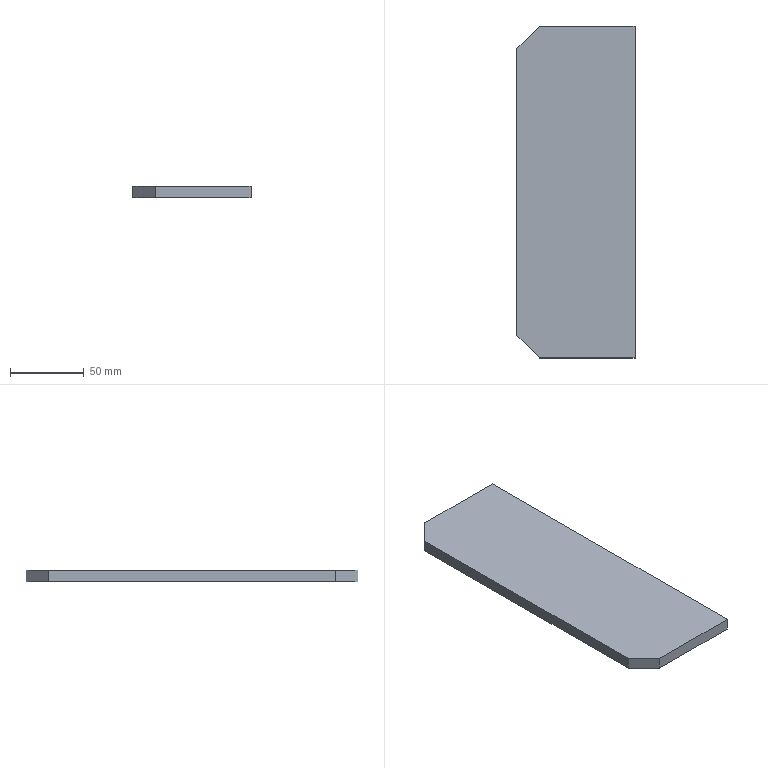Part | STEP file | 04-Rib plate | 1 solid | 8 faces | box 80 x 225 x 8 mm | volume 142200 mm3 | plane 8
STEP:
#1=CARTESIAN_POINT('',(0.,0.,0.));
#2=DIRECTION('',(0.,0.,1.));
#3=DIRECTION('',(1.,0.,0.));
#4=AXIS2_PLACEMENT_3D('',#1,#2,#3);
#5=CARTESIAN_POINT('',(0.,-225.,0.));
#6=VERTEX_POINT('',#5);
#7=CARTESIAN_POINT('',(0.,0.,0.));
#8=VERTEX_POINT('',#7);
#9=CARTESIAN_POINT('',(0.,0.,0.));
#10=DIRECTION('',(0.,1.,0.));
#11=VECTOR('',#10,1.);
#12=LINE('',#9,#11);
#13=CARTESIAN_POINT('',(0.,0.,8.));
#14=DIRECTION('',(-1.,0.,0.));
#15=DIRECTION('',(0.,-1.,0.));
#16=AXIS2_PLACEMENT_3D('',#13,#14,#15);
#17=PLANE('',#16);
#18=CARTESIAN_POINT('',(0.,-8.));
#19=DIRECTION('',(-1.,0.));
#20=VECTOR('',#19,1.);
#21=LINE('',#18,#20);
#22=(GEOMETRIC_REPRESENTATION_CONTEXT(2)PARAMETRIC_REPRESENTATION_CONTEXT()REPRESENTATION_CONTEXT('',''));
#23=DEFINITIONAL_REPRESENTATION('',(#21),#22);
#24=PCURVE('',#17,#23);
#25=CARTESIAN_POINT('',(0.,0.,0.));
#26=DIRECTION('',(0.,0.,-1.));
#27=DIRECTION('',(-1.,0.,0.));
#28=AXIS2_PLACEMENT_3D('',#25,#26,#27);
#29=PLANE('',#28);
#30=CARTESIAN_POINT('',(0.,0.));
#31=DIRECTION('',(0.,1.));
#32=VECTOR('',#31,1.);
#33=LINE('',#30,#32);
#34=(GEOMETRIC_REPRESENTATION_CONTEXT(2)PARAMETRIC_REPRESENTATION_CONTEXT()REPRESENTATION_CONTEXT('',''));
#35=DEFINITIONAL_REPRESENTATION('',(#33),#34);
#36=PCURVE('',#29,#35);
#37=SURFACE_CURVE('',#12,(#24,#36),.PCURVE_S1.);
#38=EDGE_CURVE('',#6,#8,#37,.T.);
#39=ORIENTED_EDGE('',*,*,#38,.T.);
#40=CARTESIAN_POINT('',(0.,0.,8.));
#41=VERTEX_POINT('',#40);
#42=CARTESIAN_POINT('',(0.,0.,8.));
#43=DIRECTION('',(0.,0.,-1.));
#44=VECTOR('',#43,1.);
#45=LINE('',#42,#44);
#46=CARTESIAN_POINT('',(0.,0.));
#47=DIRECTION('',(0.,-1.));
#48=VECTOR('',#47,1.);
#49=LINE('',#46,#48);
#50=(GEOMETRIC_REPRESENTATION_CONTEXT(2)PARAMETRIC_REPRESENTATION_CONTEXT()REPRESENTATION_CONTEXT('',''));
#51=DEFINITIONAL_REPRESENTATION('',(#49),#50);
#52=PCURVE('',#17,#51);
#53=CARTESIAN_POINT('',(0.,0.,8.));
#54=DIRECTION('',(0.,-1.,0.));
#55=DIRECTION('',(1.,0.,0.));
#56=AXIS2_PLACEMENT_3D('',#53,#54,#55);
#57=PLANE('',#56);
#58=CARTESIAN_POINT('',(0.,0.));
#59=DIRECTION('',(0.,-1.));
#60=VECTOR('',#59,1.);
#61=LINE('',#58,#60);
#62=(GEOMETRIC_REPRESENTATION_CONTEXT(2)PARAMETRIC_REPRESENTATION_CONTEXT()REPRESENTATION_CONTEXT('',''));
#63=DEFINITIONAL_REPRESENTATION('',(#61),#62);
#64=PCURVE('',#57,#63);
#65=SURFACE_CURVE('',#45,(#52,#64),.PCURVE_S1.);
#66=EDGE_CURVE('',#41,#8,#65,.T.);
#67=ORIENTED_EDGE('',*,*,#66,.F.);
#68=CARTESIAN_POINT('',(0.,-225.,8.));
#69=VERTEX_POINT('',#68);
#70=CARTESIAN_POINT('',(0.,0.,8.));
#71=DIRECTION('',(0.,1.,0.));
#72=VECTOR('',#71,1.);
#73=LINE('',#70,#72);
#74=CARTESIAN_POINT('',(0.,0.));
#75=DIRECTION('',(-1.,0.));
#76=VECTOR('',#75,1.);
#77=LINE('',#74,#76);
#78=(GEOMETRIC_REPRESENTATION_CONTEXT(2)PARAMETRIC_REPRESENTATION_CONTEXT()REPRESENTATION_CONTEXT('',''));
#79=DEFINITIONAL_REPRESENTATION('',(#77),#78);
#80=PCURVE('',#17,#79);
#81=CARTESIAN_POINT('',(0.,0.,8.));
#82=DIRECTION('',(0.,0.,-1.));
#83=DIRECTION('',(-1.,0.,0.));
#84=AXIS2_PLACEMENT_3D('',#81,#82,#83);
#85=PLANE('',#84);
#86=CARTESIAN_POINT('',(0.,0.));
#87=DIRECTION('',(0.,1.));
#88=VECTOR('',#87,1.);
#89=LINE('',#86,#88);
#90=(GEOMETRIC_REPRESENTATION_CONTEXT(2)PARAMETRIC_REPRESENTATION_CONTEXT()REPRESENTATION_CONTEXT('',''));
#91=DEFINITIONAL_REPRESENTATION('',(#89),#90);
#92=PCURVE('',#85,#91);
#93=SURFACE_CURVE('',#73,(#80,#92),.PCURVE_S1.);
#94=EDGE_CURVE('',#69,#41,#93,.T.);
#95=ORIENTED_EDGE('',*,*,#94,.F.);
#96=CARTESIAN_POINT('',(0.,-225.,8.));
#97=DIRECTION('',(0.,0.,-1.));
#98=VECTOR('',#97,1.);
#99=LINE('',#96,#98);
#100=CARTESIAN_POINT('',(225.,0.));
#101=DIRECTION('',(0.,-1.));
#102=VECTOR('',#101,1.);
#103=LINE('',#100,#102);
#104=(GEOMETRIC_REPRESENTATION_CONTEXT(2)PARAMETRIC_REPRESENTATION_CONTEXT()REPRESENTATION_CONTEXT('',''));
#105=DEFINITIONAL_REPRESENTATION('',(#103),#104);
#106=PCURVE('',#17,#105);
#107=CARTESIAN_POINT('',(0.,-225.,8.));
#108=DIRECTION('',(0.,1.,0.));
#109=DIRECTION('',(-1.,0.,0.));
#110=AXIS2_PLACEMENT_3D('',#107,#108,#109);
#111=PLANE('',#110);
#112=CARTESIAN_POINT('',(0.,0.));
#113=DIRECTION('',(0.,-1.));
#114=VECTOR('',#113,1.);
#115=LINE('',#112,#114);
#116=(GEOMETRIC_REPRESENTATION_CONTEXT(2)PARAMETRIC_REPRESENTATION_CONTEXT()REPRESENTATION_CONTEXT('',''));
#117=DEFINITIONAL_REPRESENTATION('',(#115),#116);
#118=PCURVE('',#111,#117);
#119=SURFACE_CURVE('',#99,(#106,#118),.PCURVE_S1.);
#120=EDGE_CURVE('',#69,#6,#119,.T.);
#121=ORIENTED_EDGE('',*,*,#120,.T.);
#122=EDGE_LOOP('',(#39,#67,#95,#121));
#123=FACE_BOUND('',#122,.T.);
#124=ADVANCED_FACE('',(#123),#17,.F.);
#125=CARTESIAN_POINT('',(-65.,0.,0.));
#126=VERTEX_POINT('',#125);
#127=CARTESIAN_POINT('',(0.,0.,0.));
#128=DIRECTION('',(-1.,0.,0.));
#129=VECTOR('',#128,1.);
#130=LINE('',#127,#129);
#131=CARTESIAN_POINT('',(0.,-8.));
#132=DIRECTION('',(-1.,0.));
#133=VECTOR('',#132,1.);
#134=LINE('',#131,#133);
#135=(GEOMETRIC_REPRESENTATION_CONTEXT(2)PARAMETRIC_REPRESENTATION_CONTEXT()REPRESENTATION_CONTEXT('',''));
#136=DEFINITIONAL_REPRESENTATION('',(#134),#135);
#137=PCURVE('',#57,#136);
#138=CARTESIAN_POINT('',(0.,0.));
#139=DIRECTION('',(1.,0.));
#140=VECTOR('',#139,1.);
#141=LINE('',#138,#140);
#142=(GEOMETRIC_REPRESENTATION_CONTEXT(2)PARAMETRIC_REPRESENTATION_CONTEXT()REPRESENTATION_CONTEXT('',''));
#143=DEFINITIONAL_REPRESENTATION('',(#141),#142);
#144=PCURVE('',#29,#143);
#145=SURFACE_CURVE('',#130,(#137,#144),.PCURVE_S1.);
#146=EDGE_CURVE('',#8,#126,#145,.T.);
#147=ORIENTED_EDGE('',*,*,#146,.T.);
#148=CARTESIAN_POINT('',(-65.,0.,8.));
#149=VERTEX_POINT('',#148);
#150=CARTESIAN_POINT('',(-65.,0.,8.));
#151=DIRECTION('',(0.,0.,-1.));
#152=VECTOR('',#151,1.);
#153=LINE('',#150,#152);
#154=CARTESIAN_POINT('',(-65.,0.));
#155=DIRECTION('',(0.,-1.));
#156=VECTOR('',#155,1.);
#157=LINE('',#154,#156);
#158=(GEOMETRIC_REPRESENTATION_CONTEXT(2)PARAMETRIC_REPRESENTATION_CONTEXT()REPRESENTATION_CONTEXT('',''));
#159=DEFINITIONAL_REPRESENTATION('',(#157),#158);
#160=PCURVE('',#57,#159);
#161=CARTESIAN_POINT('',(-65.,0.,8.));
#162=DIRECTION('',(0.7071,-0.7071,0.));
#163=DIRECTION('',(0.7071,0.7071,0.));
#164=AXIS2_PLACEMENT_3D('',#161,#162,#163);
#165=PLANE('',#164);
#166=CARTESIAN_POINT('',(0.,0.));
#167=DIRECTION('',(0.,-1.));
#168=VECTOR('',#167,1.);
#169=LINE('',#166,#168);
#170=(GEOMETRIC_REPRESENTATION_CONTEXT(2)PARAMETRIC_REPRESENTATION_CONTEXT()REPRESENTATION_CONTEXT('',''));
#171=DEFINITIONAL_REPRESENTATION('',(#169),#170);
#172=PCURVE('',#165,#171);
#173=SURFACE_CURVE('',#153,(#160,#172),.PCURVE_S1.);
#174=EDGE_CURVE('',#149,#126,#173,.T.);
#175=ORIENTED_EDGE('',*,*,#174,.F.);
#176=CARTESIAN_POINT('',(0.,0.,8.));
#177=DIRECTION('',(-1.,0.,0.));
#178=VECTOR('',#177,1.);
#179=LINE('',#176,#178);
#180=CARTESIAN_POINT('',(0.,0.));
#181=DIRECTION('',(-1.,0.));
#182=VECTOR('',#181,1.);
#183=LINE('',#180,#182);
#184=(GEOMETRIC_REPRESENTATION_CONTEXT(2)PARAMETRIC_REPRESENTATION_CONTEXT()REPRESENTATION_CONTEXT('',''));
#185=DEFINITIONAL_REPRESENTATION('',(#183),#184);
#186=PCURVE('',#57,#185);
#187=CARTESIAN_POINT('',(0.,0.));
#188=DIRECTION('',(1.,0.));
#189=VECTOR('',#188,1.);
#190=LINE('',#187,#189);
#191=(GEOMETRIC_REPRESENTATION_CONTEXT(2)PARAMETRIC_REPRESENTATION_CONTEXT()REPRESENTATION_CONTEXT('',''));
#192=DEFINITIONAL_REPRESENTATION('',(#190),#191);
#193=PCURVE('',#85,#192);
#194=SURFACE_CURVE('',#179,(#186,#193),.PCURVE_S1.);
#195=EDGE_CURVE('',#41,#149,#194,.T.);
#196=ORIENTED_EDGE('',*,*,#195,.F.);
#197=ORIENTED_EDGE('',*,*,#66,.T.);
#198=EDGE_LOOP('',(#147,#175,#196,#197));
#199=FACE_BOUND('',#198,.T.);
#200=ADVANCED_FACE('',(#199),#57,.F.);
#201=CARTESIAN_POINT('',(-80.,-15.,0.));
#202=VERTEX_POINT('',#201);
#203=CARTESIAN_POINT('',(-65.,0.,0.));
#204=DIRECTION('',(-0.7071,-0.7071,0.));
#205=VECTOR('',#204,1.);
#206=LINE('',#203,#205);
#207=CARTESIAN_POINT('',(0.,-8.));
#208=DIRECTION('',(-1.,0.));
#209=VECTOR('',#208,1.);
#210=LINE('',#207,#209);
#211=(GEOMETRIC_REPRESENTATION_CONTEXT(2)PARAMETRIC_REPRESENTATION_CONTEXT()REPRESENTATION_CONTEXT('',''));
#212=DEFINITIONAL_REPRESENTATION('',(#210),#211);
#213=PCURVE('',#165,#212);
#214=CARTESIAN_POINT('',(65.,0.));
#215=DIRECTION('',(0.7071,-0.7071));
#216=VECTOR('',#215,1.);
#217=LINE('',#214,#216);
#218=(GEOMETRIC_REPRESENTATION_CONTEXT(2)PARAMETRIC_REPRESENTATION_CONTEXT()REPRESENTATION_CONTEXT('',''));
#219=DEFINITIONAL_REPRESENTATION('',(#217),#218);
#220=PCURVE('',#29,#219);
#221=SURFACE_CURVE('',#206,(#213,#220),.PCURVE_S1.);
#222=EDGE_CURVE('',#126,#202,#221,.T.);
#223=ORIENTED_EDGE('',*,*,#222,.T.);
#224=CARTESIAN_POINT('',(-80.,-15.,8.));
#225=VERTEX_POINT('',#224);
#226=CARTESIAN_POINT('',(-80.,-15.,8.));
#227=DIRECTION('',(0.,0.,-1.));
#228=VECTOR('',#227,1.);
#229=LINE('',#226,#228);
#230=CARTESIAN_POINT('',(-21.213,0.));
#231=DIRECTION('',(0.,-1.));
#232=VECTOR('',#231,1.);
#233=LINE('',#230,#232);
#234=(GEOMETRIC_REPRESENTATION_CONTEXT(2)PARAMETRIC_REPRESENTATION_CONTEXT()REPRESENTATION_CONTEXT('',''));
#235=DEFINITIONAL_REPRESENTATION('',(#233),#234);
#236=PCURVE('',#165,#235);
#237=CARTESIAN_POINT('',(-80.,-15.,8.));
#238=DIRECTION('',(1.,0.,0.));
#239=DIRECTION('',(0.,1.,0.));
#240=AXIS2_PLACEMENT_3D('',#237,#238,#239);
#241=PLANE('',#240);
#242=CARTESIAN_POINT('',(0.,0.));
#243=DIRECTION('',(0.,-1.));
#244=VECTOR('',#243,1.);
#245=LINE('',#242,#244);
#246=(GEOMETRIC_REPRESENTATION_CONTEXT(2)PARAMETRIC_REPRESENTATION_CONTEXT()REPRESENTATION_CONTEXT('',''));
#247=DEFINITIONAL_REPRESENTATION('',(#245),#246);
#248=PCURVE('',#241,#247);
#249=SURFACE_CURVE('',#229,(#236,#248),.PCURVE_S1.);
#250=EDGE_CURVE('',#225,#202,#249,.T.);
#251=ORIENTED_EDGE('',*,*,#250,.F.);
#252=CARTESIAN_POINT('',(-65.,0.,8.));
#253=DIRECTION('',(-0.7071,-0.7071,0.));
#254=VECTOR('',#253,1.);
#255=LINE('',#252,#254);
#256=CARTESIAN_POINT('',(0.,0.));
#257=DIRECTION('',(-1.,0.));
#258=VECTOR('',#257,1.);
#259=LINE('',#256,#258);
#260=(GEOMETRIC_REPRESENTATION_CONTEXT(2)PARAMETRIC_REPRESENTATION_CONTEXT()REPRESENTATION_CONTEXT('',''));
#261=DEFINITIONAL_REPRESENTATION('',(#259),#260);
#262=PCURVE('',#165,#261);
#263=CARTESIAN_POINT('',(65.,0.));
#264=DIRECTION('',(0.7071,-0.7071));
#265=VECTOR('',#264,1.);
#266=LINE('',#263,#265);
#267=(GEOMETRIC_REPRESENTATION_CONTEXT(2)PARAMETRIC_REPRESENTATION_CONTEXT()REPRESENTATION_CONTEXT('',''));
#268=DEFINITIONAL_REPRESENTATION('',(#266),#267);
#269=PCURVE('',#85,#268);
#270=SURFACE_CURVE('',#255,(#262,#269),.PCURVE_S1.);
#271=EDGE_CURVE('',#149,#225,#270,.T.);
#272=ORIENTED_EDGE('',*,*,#271,.F.);
#273=ORIENTED_EDGE('',*,*,#174,.T.);
#274=EDGE_LOOP('',(#223,#251,#272,#273));
#275=FACE_BOUND('',#274,.T.);
#276=ADVANCED_FACE('',(#275),#165,.F.);
#277=CARTESIAN_POINT('',(-80.,-210.,0.));
#278=VERTEX_POINT('',#277);
#279=CARTESIAN_POINT('',(-80.,-15.,0.));
#280=DIRECTION('',(0.,-1.,0.));
#281=VECTOR('',#280,1.);
#282=LINE('',#279,#281);
#283=CARTESIAN_POINT('',(0.,-8.));
#284=DIRECTION('',(-1.,0.));
#285=VECTOR('',#284,1.);
#286=LINE('',#283,#285);
#287=(GEOMETRIC_REPRESENTATION_CONTEXT(2)PARAMETRIC_REPRESENTATION_CONTEXT()REPRESENTATION_CONTEXT('',''));
#288=DEFINITIONAL_REPRESENTATION('',(#286),#287);
#289=PCURVE('',#241,#288);
#290=CARTESIAN_POINT('',(80.,-15.));
#291=DIRECTION('',(0.,-1.));
#292=VECTOR('',#291,1.);
#293=LINE('',#290,#292);
#294=(GEOMETRIC_REPRESENTATION_CONTEXT(2)PARAMETRIC_REPRESENTATION_CONTEXT()REPRESENTATION_CONTEXT('',''));
#295=DEFINITIONAL_REPRESENTATION('',(#293),#294);
#296=PCURVE('',#29,#295);
#297=SURFACE_CURVE('',#282,(#289,#296),.PCURVE_S1.);
#298=EDGE_CURVE('',#202,#278,#297,.T.);
#299=ORIENTED_EDGE('',*,*,#298,.T.);
#300=CARTESIAN_POINT('',(-80.,-210.,8.));
#301=VERTEX_POINT('',#300);
#302=CARTESIAN_POINT('',(-80.,-210.,8.));
#303=DIRECTION('',(0.,0.,-1.));
#304=VECTOR('',#303,1.);
#305=LINE('',#302,#304);
#306=CARTESIAN_POINT('',(-195.,0.));
#307=DIRECTION('',(0.,-1.));
#308=VECTOR('',#307,1.);
#309=LINE('',#306,#308);
#310=(GEOMETRIC_REPRESENTATION_CONTEXT(2)PARAMETRIC_REPRESENTATION_CONTEXT()REPRESENTATION_CONTEXT('',''));
#311=DEFINITIONAL_REPRESENTATION('',(#309),#310);
#312=PCURVE('',#241,#311);
#313=CARTESIAN_POINT('',(-80.,-210.,8.));
#314=DIRECTION('',(0.7071,0.7071,0.));
#315=DIRECTION('',(-0.7071,0.7071,0.));
#316=AXIS2_PLACEMENT_3D('',#313,#314,#315);
#317=PLANE('',#316);
#318=CARTESIAN_POINT('',(0.,0.));
#319=DIRECTION('',(0.,-1.));
#320=VECTOR('',#319,1.);
#321=LINE('',#318,#320);
#322=(GEOMETRIC_REPRESENTATION_CONTEXT(2)PARAMETRIC_REPRESENTATION_CONTEXT()REPRESENTATION_CONTEXT('',''));
#323=DEFINITIONAL_REPRESENTATION('',(#321),#322);
#324=PCURVE('',#317,#323);
#325=SURFACE_CURVE('',#305,(#312,#324),.PCURVE_S1.);
#326=EDGE_CURVE('',#301,#278,#325,.T.);
#327=ORIENTED_EDGE('',*,*,#326,.F.);
#328=CARTESIAN_POINT('',(-80.,-15.,8.));
#329=DIRECTION('',(0.,-1.,0.));
#330=VECTOR('',#329,1.);
#331=LINE('',#328,#330);
#332=CARTESIAN_POINT('',(0.,0.));
#333=DIRECTION('',(-1.,0.));
#334=VECTOR('',#333,1.);
#335=LINE('',#332,#334);
#336=(GEOMETRIC_REPRESENTATION_CONTEXT(2)PARAMETRIC_REPRESENTATION_CONTEXT()REPRESENTATION_CONTEXT('',''));
#337=DEFINITIONAL_REPRESENTATION('',(#335),#336);
#338=PCURVE('',#241,#337);
#339=CARTESIAN_POINT('',(80.,-15.));
#340=DIRECTION('',(0.,-1.));
#341=VECTOR('',#340,1.);
#342=LINE('',#339,#341);
#343=(GEOMETRIC_REPRESENTATION_CONTEXT(2)PARAMETRIC_REPRESENTATION_CONTEXT()REPRESENTATION_CONTEXT('',''));
#344=DEFINITIONAL_REPRESENTATION('',(#342),#343);
#345=PCURVE('',#85,#344);
#346=SURFACE_CURVE('',#331,(#338,#345),.PCURVE_S1.);
#347=EDGE_CURVE('',#225,#301,#346,.T.);
#348=ORIENTED_EDGE('',*,*,#347,.F.);
#349=ORIENTED_EDGE('',*,*,#250,.T.);
#350=EDGE_LOOP('',(#299,#327,#348,#349));
#351=FACE_BOUND('',#350,.T.);
#352=ADVANCED_FACE('',(#351),#241,.F.);
#353=CARTESIAN_POINT('',(-65.,-225.,0.));
#354=VERTEX_POINT('',#353);
#355=CARTESIAN_POINT('',(-80.,-210.,0.));
#356=DIRECTION('',(0.7071,-0.7071,0.));
#357=VECTOR('',#356,1.);
#358=LINE('',#355,#357);
#359=CARTESIAN_POINT('',(0.,-8.));
#360=DIRECTION('',(-1.,0.));
#361=VECTOR('',#360,1.);
#362=LINE('',#359,#361);
#363=(GEOMETRIC_REPRESENTATION_CONTEXT(2)PARAMETRIC_REPRESENTATION_CONTEXT()REPRESENTATION_CONTEXT('',''));
#364=DEFINITIONAL_REPRESENTATION('',(#362),#363);
#365=PCURVE('',#317,#364);
#366=CARTESIAN_POINT('',(80.,-210.));
#367=DIRECTION('',(-0.7071,-0.7071));
#368=VECTOR('',#367,1.);
#369=LINE('',#366,#368);
#370=(GEOMETRIC_REPRESENTATION_CONTEXT(2)PARAMETRIC_REPRESENTATION_CONTEXT()REPRESENTATION_CONTEXT('',''));
#371=DEFINITIONAL_REPRESENTATION('',(#369),#370);
#372=PCURVE('',#29,#371);
#373=SURFACE_CURVE('',#358,(#365,#372),.PCURVE_S1.);
#374=EDGE_CURVE('',#278,#354,#373,.T.);
#375=ORIENTED_EDGE('',*,*,#374,.T.);
#376=CARTESIAN_POINT('',(-65.,-225.,8.));
#377=VERTEX_POINT('',#376);
#378=CARTESIAN_POINT('',(-65.,-225.,8.));
#379=DIRECTION('',(0.,0.,-1.));
#380=VECTOR('',#379,1.);
#381=LINE('',#378,#380);
#382=CARTESIAN_POINT('',(-21.213,0.));
#383=DIRECTION('',(0.,-1.));
#384=VECTOR('',#383,1.);
#385=LINE('',#382,#384);
#386=(GEOMETRIC_REPRESENTATION_CONTEXT(2)PARAMETRIC_REPRESENTATION_CONTEXT()REPRESENTATION_CONTEXT('',''));
#387=DEFINITIONAL_REPRESENTATION('',(#385),#386);
#388=PCURVE('',#317,#387);
#389=CARTESIAN_POINT('',(65.,0.));
#390=DIRECTION('',(0.,-1.));
#391=VECTOR('',#390,1.);
#392=LINE('',#389,#391);
#393=(GEOMETRIC_REPRESENTATION_CONTEXT(2)PARAMETRIC_REPRESENTATION_CONTEXT()REPRESENTATION_CONTEXT('',''));
#394=DEFINITIONAL_REPRESENTATION('',(#392),#393);
#395=PCURVE('',#111,#394);
#396=SURFACE_CURVE('',#381,(#388,#395),.PCURVE_S1.);
#397=EDGE_CURVE('',#377,#354,#396,.T.);
#398=ORIENTED_EDGE('',*,*,#397,.F.);
#399=CARTESIAN_POINT('',(-80.,-210.,8.));
#400=DIRECTION('',(0.7071,-0.7071,0.));
#401=VECTOR('',#400,1.);
#402=LINE('',#399,#401);
#403=CARTESIAN_POINT('',(0.,0.));
#404=DIRECTION('',(-1.,0.));
#405=VECTOR('',#404,1.);
#406=LINE('',#403,#405);
#407=(GEOMETRIC_REPRESENTATION_CONTEXT(2)PARAMETRIC_REPRESENTATION_CONTEXT()REPRESENTATION_CONTEXT('',''));
#408=DEFINITIONAL_REPRESENTATION('',(#406),#407);
#409=PCURVE('',#317,#408);
#410=CARTESIAN_POINT('',(80.,-210.));
#411=DIRECTION('',(-0.7071,-0.7071));
#412=VECTOR('',#411,1.);
#413=LINE('',#410,#412);
#414=(GEOMETRIC_REPRESENTATION_CONTEXT(2)PARAMETRIC_REPRESENTATION_CONTEXT()REPRESENTATION_CONTEXT('',''));
#415=DEFINITIONAL_REPRESENTATION('',(#413),#414);
#416=PCURVE('',#85,#415);
#417=SURFACE_CURVE('',#402,(#409,#416),.PCURVE_S1.);
#418=EDGE_CURVE('',#301,#377,#417,.T.);
#419=ORIENTED_EDGE('',*,*,#418,.F.);
#420=ORIENTED_EDGE('',*,*,#326,.T.);
#421=EDGE_LOOP('',(#375,#398,#419,#420));
#422=FACE_BOUND('',#421,.T.);
#423=ADVANCED_FACE('',(#422),#317,.F.);
#424=CARTESIAN_POINT('',(0.,-225.,0.));
#425=DIRECTION('',(1.,0.,0.));
#426=VECTOR('',#425,1.);
#427=LINE('',#424,#426);
#428=CARTESIAN_POINT('',(0.,-8.));
#429=DIRECTION('',(-1.,0.));
#430=VECTOR('',#429,1.);
#431=LINE('',#428,#430);
#432=(GEOMETRIC_REPRESENTATION_CONTEXT(2)PARAMETRIC_REPRESENTATION_CONTEXT()REPRESENTATION_CONTEXT('',''));
#433=DEFINITIONAL_REPRESENTATION('',(#431),#432);
#434=PCURVE('',#111,#433);
#435=CARTESIAN_POINT('',(0.,-225.));
#436=DIRECTION('',(-1.,0.));
#437=VECTOR('',#436,1.);
#438=LINE('',#435,#437);
#439=(GEOMETRIC_REPRESENTATION_CONTEXT(2)PARAMETRIC_REPRESENTATION_CONTEXT()REPRESENTATION_CONTEXT('',''));
#440=DEFINITIONAL_REPRESENTATION('',(#438),#439);
#441=PCURVE('',#29,#440);
#442=SURFACE_CURVE('',#427,(#434,#441),.PCURVE_S1.);
#443=EDGE_CURVE('',#354,#6,#442,.T.);
#444=ORIENTED_EDGE('',*,*,#443,.T.);
#445=ORIENTED_EDGE('',*,*,#120,.F.);
#446=CARTESIAN_POINT('',(0.,-225.,8.));
#447=DIRECTION('',(1.,0.,0.));
#448=VECTOR('',#447,1.);
#449=LINE('',#446,#448);
#450=CARTESIAN_POINT('',(0.,0.));
#451=DIRECTION('',(-1.,0.));
#452=VECTOR('',#451,1.);
#453=LINE('',#450,#452);
#454=(GEOMETRIC_REPRESENTATION_CONTEXT(2)PARAMETRIC_REPRESENTATION_CONTEXT()REPRESENTATION_CONTEXT('',''));
#455=DEFINITIONAL_REPRESENTATION('',(#453),#454);
#456=PCURVE('',#111,#455);
#457=CARTESIAN_POINT('',(0.,-225.));
#458=DIRECTION('',(-1.,0.));
#459=VECTOR('',#458,1.);
#460=LINE('',#457,#459);
#461=(GEOMETRIC_REPRESENTATION_CONTEXT(2)PARAMETRIC_REPRESENTATION_CONTEXT()REPRESENTATION_CONTEXT('',''));
#462=DEFINITIONAL_REPRESENTATION('',(#460),#461);
#463=PCURVE('',#85,#462);
#464=SURFACE_CURVE('',#449,(#456,#463),.PCURVE_S1.);
#465=EDGE_CURVE('',#377,#69,#464,.T.);
#466=ORIENTED_EDGE('',*,*,#465,.F.);
#467=ORIENTED_EDGE('',*,*,#397,.T.);
#468=EDGE_LOOP('',(#444,#445,#466,#467));
#469=FACE_BOUND('',#468,.T.);
#470=ADVANCED_FACE('',(#469),#111,.F.);
#471=ORIENTED_EDGE('',*,*,#94,.T.);
#472=ORIENTED_EDGE('',*,*,#195,.T.);
#473=ORIENTED_EDGE('',*,*,#271,.T.);
#474=ORIENTED_EDGE('',*,*,#347,.T.);
#475=ORIENTED_EDGE('',*,*,#418,.T.);
#476=ORIENTED_EDGE('',*,*,#465,.T.);
#477=EDGE_LOOP('',(#471,#472,#473,#474,#475,#476));
#478=FACE_BOUND('',#477,.T.);
#479=ADVANCED_FACE('',(#478),#85,.F.);
#480=ORIENTED_EDGE('',*,*,#38,.F.);
#481=ORIENTED_EDGE('',*,*,#443,.F.);
#482=ORIENTED_EDGE('',*,*,#374,.F.);
#483=ORIENTED_EDGE('',*,*,#298,.F.);
#484=ORIENTED_EDGE('',*,*,#222,.F.);
#485=ORIENTED_EDGE('',*,*,#146,.F.);
#486=EDGE_LOOP('',(#480,#481,#482,#483,#484,#485));
#487=FACE_BOUND('',#486,.T.);
#488=ADVANCED_FACE('',(#487),#29,.T.);
#489=CLOSED_SHELL('',(#124,#200,#276,#352,#423,#470,#479,#488));
#490=MANIFOLD_SOLID_BREP('',#489);
#491=(LENGTH_UNIT()NAMED_UNIT(*)SI_UNIT(.MILLI.,.METRE.));
#492=UNCERTAINTY_MEASURE_WITH_UNIT(LENGTH_MEASURE(0.0000001),#491,'','');
#493=(NAMED_UNIT(*)PLANE_ANGLE_UNIT()SI_UNIT($,.RADIAN.));
#494=(NAMED_UNIT(*)SI_UNIT($,.STERADIAN.)SOLID_ANGLE_UNIT());
#495=(GEOMETRIC_REPRESENTATION_CONTEXT(3)GLOBAL_UNCERTAINTY_ASSIGNED_CONTEXT((#492))GLOBAL_UNIT_ASSIGNED_CONTEXT((#491,#493,#494))REPRESENTATION_CONTEXT('',''));
#496=ADVANCED_BREP_SHAPE_REPRESENTATION('',(#4,#490),#495);